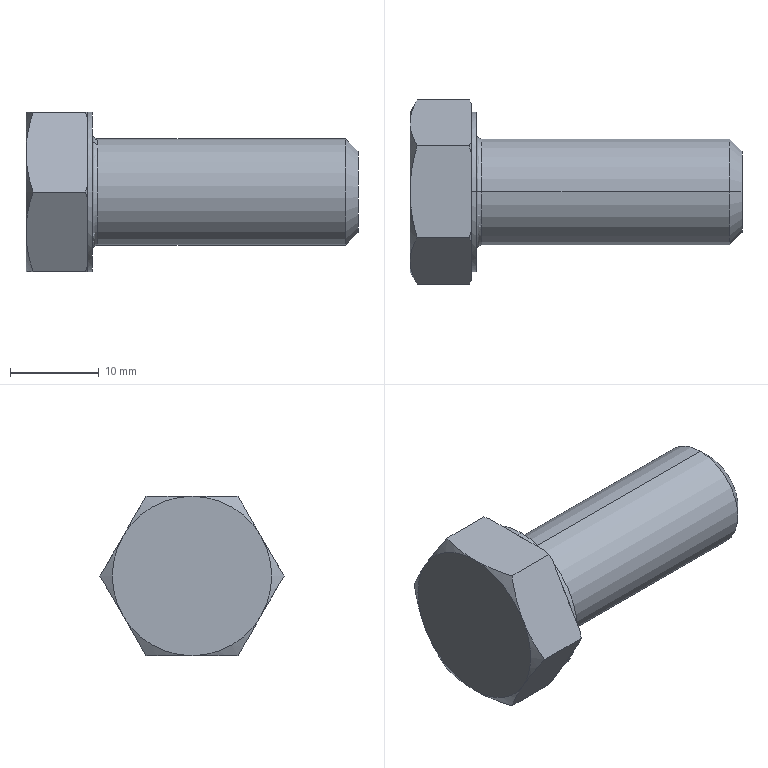Part | SolidWorks | features RevCut 4, Chamfer 1, Extrusion 1, Fillet 1, LPattern 1, Revolution 1 | 1 solid | 35 faces | box 37.5 x 20.785 x 18 mm | volume 5444 mm3 | plane 15 | cone 14 | cylinder 4 | torus 2 | commonest cylinder face diameters 12 x2 18 x2
STEP:
#1=CARTESIAN_POINT('',(8.1,0.,6.));
#2=VERTEX_POINT('',#1);
#3=CARTESIAN_POINT('',(8.1,0.,-6.));
#4=VERTEX_POINT('',#3);
#5=CARTESIAN_POINT('',(8.1,0.,0.));
#6=DIRECTION('',(1.,0.,0.));
#7=DIRECTION('',(0.,0.,-1.));
#8=AXIS2_PLACEMENT_3D('',#5,#6,#7);
#9=CIRCLE('',#8,6.);
#10=EDGE_CURVE('',#2,#4,#9,.T.);
#11=ORIENTED_EDGE('',*,*,#10,.F.);
#12=CARTESIAN_POINT('',(7.5,0.,6.6));
#13=VERTEX_POINT('',#12);
#14=CARTESIAN_POINT('',(8.1,0.,6.6));
#15=DIRECTION('',(0.,1.,0.));
#16=DIRECTION('',(0.,0.,1.));
#17=AXIS2_PLACEMENT_3D('',#14,#15,#16);
#18=CIRCLE('',#17,0.6);
#19=EDGE_CURVE('',#2,#13,#18,.T.);
#20=ORIENTED_EDGE('',*,*,#19,.T.);
#21=CARTESIAN_POINT('',(7.5,0.,-6.6));
#22=VERTEX_POINT('',#21);
#23=CARTESIAN_POINT('',(7.5,0.,0.));
#24=DIRECTION('',(-1.,0.,0.));
#25=DIRECTION('',(0.,0.,-1.));
#26=AXIS2_PLACEMENT_3D('',#23,#24,#25);
#27=CIRCLE('',#26,6.6);
#28=EDGE_CURVE('',#22,#13,#27,.T.);
#29=ORIENTED_EDGE('',*,*,#28,.F.);
#30=CARTESIAN_POINT('',(8.1,0.,-6.6));
#31=DIRECTION('',(0.,-1.,0.));
#32=DIRECTION('',(0.,0.,-1.));
#33=AXIS2_PLACEMENT_3D('',#30,#31,#32);
#34=CIRCLE('',#33,0.6);
#35=EDGE_CURVE('',#4,#22,#34,.T.);
#36=ORIENTED_EDGE('',*,*,#35,.F.);
#37=EDGE_LOOP('',(#11,#20,#29,#36));
#38=FACE_OUTER_BOUND('',#37,.T.);
#39=CARTESIAN_POINT('',(8.1,0.,0.));
#40=DIRECTION('',(1.,0.,0.));
#41=DIRECTION('',(0.,0.,-1.));
#42=AXIS2_PLACEMENT_3D('',#39,#40,#41);
#43=TOROIDAL_SURFACE('',#42,6.6,0.6);
#44=ADVANCED_FACE('',(#38),#43,.F.);
#45=CARTESIAN_POINT('',(37.5,0.,-4.6));
#46=VERTEX_POINT('',#45);
#47=CARTESIAN_POINT('',(37.5,0.,4.6));
#48=VERTEX_POINT('',#47);
#49=CARTESIAN_POINT('',(37.5,0.,0.));
#50=DIRECTION('',(1.,0.,0.));
#51=DIRECTION('',(0.,0.,1.));
#52=AXIS2_PLACEMENT_3D('',#49,#50,#51);
#53=CIRCLE('',#52,4.6);
#54=EDGE_CURVE('',#46,#48,#53,.T.);
#55=ORIENTED_EDGE('',*,*,#54,.F.);
#56=CARTESIAN_POINT('',(36.1,0.,-6.));
#57=VERTEX_POINT('',#56);
#58=CARTESIAN_POINT('',(36.1,0.,-6.));
#59=DIRECTION('',(-0.7071,0.,-0.7071));
#60=VECTOR('',#59,1000.);
#61=LINE('',#58,#60);
#62=EDGE_CURVE('',#46,#57,#61,.T.);
#63=ORIENTED_EDGE('',*,*,#62,.T.);
#64=CARTESIAN_POINT('',(36.1,0.,6.));
#65=VERTEX_POINT('',#64);
#66=CARTESIAN_POINT('',(36.1,0.,0.));
#67=DIRECTION('',(-1.,0.,0.));
#68=DIRECTION('',(0.,0.,1.));
#69=AXIS2_PLACEMENT_3D('',#66,#67,#68);
#70=CIRCLE('',#69,6.);
#71=EDGE_CURVE('',#65,#57,#70,.T.);
#72=ORIENTED_EDGE('',*,*,#71,.F.);
#73=CARTESIAN_POINT('',(36.1,0.,6.));
#74=DIRECTION('',(-0.7071,0.,0.7071));
#75=VECTOR('',#74,1000.);
#76=LINE('',#73,#75);
#77=EDGE_CURVE('',#48,#65,#76,.T.);
#78=ORIENTED_EDGE('',*,*,#77,.F.);
#79=EDGE_LOOP('',(#55,#63,#72,#78));
#80=FACE_OUTER_BOUND('',#79,.T.);
#81=CARTESIAN_POINT('',(36.1,0.,0.));
#82=DIRECTION('',(-1.,0.,0.));
#83=DIRECTION('',(0.,0.,1.));
#84=AXIS2_PLACEMENT_3D('',#81,#82,#83);
#85=CONICAL_SURFACE('',#84,6.,0.7854);
#86=ADVANCED_FACE('',(#80),#85,.T.);
#87=ORIENTED_EDGE('',*,*,#71,.T.);
#88=CARTESIAN_POINT('',(0.,0.,-6.));
#89=DIRECTION('',(-1.,0.,0.));
#90=VECTOR('',#89,1000.);
#91=LINE('',#88,#90);
#92=EDGE_CURVE('',#57,#4,#91,.T.);
#93=ORIENTED_EDGE('',*,*,#92,.T.);
#94=CARTESIAN_POINT('',(8.1,0.,0.));
#95=DIRECTION('',(1.,0.,0.));
#96=DIRECTION('',(0.,0.,-1.));
#97=AXIS2_PLACEMENT_3D('',#94,#95,#96);
#98=CIRCLE('',#97,6.);
#99=EDGE_CURVE('',#4,#2,#98,.T.);
#100=ORIENTED_EDGE('',*,*,#99,.T.);
#101=CARTESIAN_POINT('',(0.,0.,6.));
#102=DIRECTION('',(-1.,0.,0.));
#103=VECTOR('',#102,1000.);
#104=LINE('',#101,#103);
#105=EDGE_CURVE('',#65,#2,#104,.T.);
#106=ORIENTED_EDGE('',*,*,#105,.F.);
#107=EDGE_LOOP('',(#87,#93,#100,#106));
#108=FACE_OUTER_BOUND('',#107,.T.);
#109=CARTESIAN_POINT('',(0.,0.,0.));
#110=DIRECTION('',(-1.,0.,0.));
#111=DIRECTION('',(0.,0.,1.));
#112=AXIS2_PLACEMENT_3D('',#109,#110,#111);
#113=CYLINDRICAL_SURFACE('',#112,6.);
#114=ADVANCED_FACE('',(#108),#113,.T.);
#115=CARTESIAN_POINT('',(7.5,0.,-9.));
#116=VERTEX_POINT('',#115);
#117=CARTESIAN_POINT('',(7.5,0.,9.));
#118=VERTEX_POINT('',#117);
#119=CARTESIAN_POINT('',(7.5,0.,0.));
#120=DIRECTION('',(1.,0.,0.));
#121=DIRECTION('',(0.,0.,-1.));
#122=AXIS2_PLACEMENT_3D('',#119,#120,#121);
#123=CIRCLE('',#122,9.);
#124=EDGE_CURVE('',#116,#118,#123,.T.);
#125=ORIENTED_EDGE('',*,*,#124,.F.);
#126=CARTESIAN_POINT('',(6.9,0.,-9.));
#127=VERTEX_POINT('',#126);
#128=CARTESIAN_POINT('',(0.,0.,-9.));
#129=DIRECTION('',(-1.,0.,0.));
#130=VECTOR('',#129,1000.);
#131=LINE('',#128,#130);
#132=EDGE_CURVE('',#116,#127,#131,.T.);
#133=ORIENTED_EDGE('',*,*,#132,.T.);
#134=CARTESIAN_POINT('',(6.9,7.794,-4.5));
#135=VERTEX_POINT('',#134);
#136=CARTESIAN_POINT('',(6.9,0.,0.));
#137=DIRECTION('',(-1.,0.,0.));
#138=DIRECTION('',(0.,0.,1.));
#139=AXIS2_PLACEMENT_3D('',#136,#137,#138);
#140=CIRCLE('',#139,9.);
#141=EDGE_CURVE('',#135,#127,#140,.T.);
#142=ORIENTED_EDGE('',*,*,#141,.F.);
#143=CARTESIAN_POINT('',(6.9,7.794,4.5));
#144=VERTEX_POINT('',#143);
#145=CARTESIAN_POINT('',(6.9,0.,0.));
#146=DIRECTION('',(-1.,0.,0.));
#147=DIRECTION('',(0.,0.,1.));
#148=AXIS2_PLACEMENT_3D('',#145,#146,#147);
#149=CIRCLE('',#148,9.);
#150=EDGE_CURVE('',#144,#135,#149,.T.);
#151=ORIENTED_EDGE('',*,*,#150,.F.);
#152=CARTESIAN_POINT('',(6.9,0.,9.));
#153=VERTEX_POINT('',#152);
#154=CARTESIAN_POINT('',(6.9,0.,0.));
#155=DIRECTION('',(-1.,0.,0.));
#156=DIRECTION('',(0.,0.,1.));
#157=AXIS2_PLACEMENT_3D('',#154,#155,#156);
#158=CIRCLE('',#157,9.);
#159=EDGE_CURVE('',#153,#144,#158,.T.);
#160=ORIENTED_EDGE('',*,*,#159,.F.);
#161=CARTESIAN_POINT('',(0.,0.,9.));
#162=DIRECTION('',(-1.,0.,0.));
#163=VECTOR('',#162,1000.);
#164=LINE('',#161,#163);
#165=EDGE_CURVE('',#118,#153,#164,.T.);
#166=ORIENTED_EDGE('',*,*,#165,.F.);
#167=EDGE_LOOP('',(#125,#133,#142,#151,#160,#166));
#168=FACE_OUTER_BOUND('',#167,.T.);
#169=CARTESIAN_POINT('',(0.,0.,0.));
#170=DIRECTION('',(-1.,0.,0.));
#171=DIRECTION('',(0.,0.,1.));
#172=AXIS2_PLACEMENT_3D('',#169,#170,#171);
#173=CYLINDRICAL_SURFACE('',#172,9.);
#174=ADVANCED_FACE('',(#168),#173,.T.);
#175=CARTESIAN_POINT('',(6.9,5.57,-8.352));
#176=VERTEX_POINT('',#175);
#177=CARTESIAN_POINT('',(6.9,5.196,-9.));
#178=DIRECTION('',(0.,0.5,0.866));
#179=VECTOR('',#178,1000.);
#180=LINE('',#177,#179);
#181=EDGE_CURVE('',#176,#135,#180,.T.);
#182=ORIENTED_EDGE('',*,*,#181,.F.);
#183=CARTESIAN_POINT('',(6.696,5.196,-9.));
#184=VERTEX_POINT('',#183);
#185=CARTESIAN_POINT('',(6.696,5.196,-9.));
#186=CARTESIAN_POINT('',(6.768,5.321,-8.785));
#187=CARTESIAN_POINT('',(6.836,5.445,-8.569));
#188=CARTESIAN_POINT('',(6.9,5.57,-8.352));
#189=B_SPLINE_CURVE_WITH_KNOTS('',3,(#185,#186,#187,#188),.UNSPECIFIED.,.F.,.F.,(4,4),(0.000000238,0.0007696),.UNSPECIFIED.);
#190=EDGE_CURVE('',#184,#176,#189,.T.);
#191=ORIENTED_EDGE('',*,*,#190,.F.);
#192=CARTESIAN_POINT('',(0.8038,5.196,-9.));
#193=VERTEX_POINT('',#192);
#194=CARTESIAN_POINT('',(7.5,5.196,-9.));
#195=DIRECTION('',(-1.,0.,0.));
#196=VECTOR('',#195,1000.);
#197=LINE('',#194,#196);
#198=EDGE_CURVE('',#184,#193,#197,.T.);
#199=ORIENTED_EDGE('',*,*,#198,.T.);
#200=CARTESIAN_POINT('',(0.,7.794,-4.5));
#201=VERTEX_POINT('',#200);
#202=CARTESIAN_POINT('',(0.,7.794,-4.5));
#203=CARTESIAN_POINT('',(0.,7.574,-4.882));
#204=CARTESIAN_POINT('',(0.019,7.352,-5.266));
#205=CARTESIAN_POINT('',(0.09253,6.914,-6.024));
#206=CARTESIAN_POINT('',(0.147,6.697,-6.401));
#207=CARTESIAN_POINT('',(0.357,6.048,-7.525));
#208=CARTESIAN_POINT('',(0.5591,5.62,-8.266));
#209=CARTESIAN_POINT('',(0.8038,5.196,-9.));
#210=B_SPLINE_CURVE_WITH_KNOTS('',3,(#202,#203,#204,#205,#206,#207,#208,#209),.UNSPECIFIED.,.F.,.F.,(4,2,2,4),(0.005258,0.006567,0.007877,0.0105),.UNSPECIFIED.);
#211=EDGE_CURVE('',#201,#193,#210,.T.);
#212=ORIENTED_EDGE('',*,*,#211,.F.);
#213=CARTESIAN_POINT('',(0.8038,10.392,0.));
#214=VERTEX_POINT('',#213);
#215=CARTESIAN_POINT('',(0.8038,10.392,0.));
#216=CARTESIAN_POINT('',(0.5585,9.967,-0.7361));
#217=CARTESIAN_POINT('',(0.3563,9.539,-1.478));
#218=CARTESIAN_POINT('',(0.07661,8.674,-2.976));
#219=CARTESIAN_POINT('',(0.,8.237,-3.733));
#220=CARTESIAN_POINT('',(0.,7.794,-4.5));
#221=B_SPLINE_CURVE_WITH_KNOTS('',3,(#215,#216,#217,#218,#219,#220),.UNSPECIFIED.,.F.,.F.,(4,2,4),(0.000000238,0.002629,0.005258),.UNSPECIFIED.);
#222=EDGE_CURVE('',#214,#201,#221,.T.);
#223=ORIENTED_EDGE('',*,*,#222,.F.);
#224=CARTESIAN_POINT('',(6.696,10.392,0.));
#225=VERTEX_POINT('',#224);
#226=CARTESIAN_POINT('',(7.5,10.392,0.));
#227=DIRECTION('',(-1.,0.,0.));
#228=VECTOR('',#227,1000.);
#229=LINE('',#226,#228);
#230=EDGE_CURVE('',#225,#214,#229,.T.);
#231=ORIENTED_EDGE('',*,*,#230,.F.);
#232=CARTESIAN_POINT('',(6.9,10.018,-0.6478));
#233=VERTEX_POINT('',#232);
#234=CARTESIAN_POINT('',(6.9,10.018,-0.6478));
#235=CARTESIAN_POINT('',(6.836,10.143,-0.4313));
#236=CARTESIAN_POINT('',(6.768,10.268,-0.2154));
#237=CARTESIAN_POINT('',(6.696,10.392,0.));
#238=B_SPLINE_CURVE_WITH_KNOTS('',3,(#234,#235,#236,#237),.UNSPECIFIED.,.F.,.F.,(4,4),(0.009728,0.0105),.UNSPECIFIED.);
#239=EDGE_CURVE('',#233,#225,#238,.T.);
#240=ORIENTED_EDGE('',*,*,#239,.F.);
#241=CARTESIAN_POINT('',(6.9,5.196,-9.));
#242=DIRECTION('',(0.,0.5,0.866));
#243=VECTOR('',#242,1000.);
#244=LINE('',#241,#243);
#245=EDGE_CURVE('',#135,#233,#244,.T.);
#246=ORIENTED_EDGE('',*,*,#245,.F.);
#247=EDGE_LOOP('',(#182,#191,#199,#212,#223,#231,#240,#246));
#248=FACE_OUTER_BOUND('',#247,.T.);
#249=CARTESIAN_POINT('',(7.5,5.196,-9.));
#250=DIRECTION('',(0.,-0.866,0.5));
#251=DIRECTION('',(0.,-0.5,-0.866));
#252=AXIS2_PLACEMENT_3D('',#249,#250,#251);
#253=PLANE('',#252);
#254=ADVANCED_FACE('',(#248),#253,.F.);
#255=CARTESIAN_POINT('',(6.9,10.018,0.6478));
#256=VERTEX_POINT('',#255);
#257=CARTESIAN_POINT('',(6.9,10.392,0.));
#258=DIRECTION('',(0.,-0.5,0.866));
#259=VECTOR('',#258,1000.);
#260=LINE('',#257,#259);
#261=EDGE_CURVE('',#256,#144,#260,.T.);
#262=ORIENTED_EDGE('',*,*,#261,.F.);
#263=CARTESIAN_POINT('',(6.696,10.392,0.));
#264=CARTESIAN_POINT('',(6.768,10.268,0.2154));
#265=CARTESIAN_POINT('',(6.836,10.143,0.4314));
#266=CARTESIAN_POINT('',(6.9,10.018,0.6478));
#267=B_SPLINE_CURVE_WITH_KNOTS('',3,(#263,#264,#265,#266),.UNSPECIFIED.,.F.,.F.,(4,4),(0.000000238,0.0007696),.UNSPECIFIED.);
#268=EDGE_CURVE('',#225,#256,#267,.T.);
#269=ORIENTED_EDGE('',*,*,#268,.F.);
#270=ORIENTED_EDGE('',*,*,#230,.T.);
#271=CARTESIAN_POINT('',(0.,7.794,4.5));
#272=VERTEX_POINT('',#271);
#273=CARTESIAN_POINT('',(0.,7.794,4.5));
#274=CARTESIAN_POINT('',(0.,8.015,4.118));
#275=CARTESIAN_POINT('',(0.019,8.236,3.734));
#276=CARTESIAN_POINT('',(0.09253,8.674,2.976));
#277=CARTESIAN_POINT('',(0.147,8.892,2.599));
#278=CARTESIAN_POINT('',(0.357,9.541,1.475));
#279=CARTESIAN_POINT('',(0.5591,9.968,0.7343));
#280=CARTESIAN_POINT('',(0.8038,10.392,0.));
#281=B_SPLINE_CURVE_WITH_KNOTS('',3,(#273,#274,#275,#276,#277,#278,#279,#280),.UNSPECIFIED.,.F.,.F.,(4,2,2,4),(0.005258,0.006567,0.007877,0.0105),.UNSPECIFIED.);
#282=EDGE_CURVE('',#272,#214,#281,.T.);
#283=ORIENTED_EDGE('',*,*,#282,.F.);
#284=CARTESIAN_POINT('',(0.8038,5.196,9.));
#285=VERTEX_POINT('',#284);
#286=CARTESIAN_POINT('',(0.8038,5.196,9.));
#287=CARTESIAN_POINT('',(0.5585,5.621,8.264));
#288=CARTESIAN_POINT('',(0.3563,6.049,7.522));
#289=CARTESIAN_POINT('',(0.07661,6.914,6.024));
#290=CARTESIAN_POINT('',(0.,7.352,5.267));
#291=CARTESIAN_POINT('',(0.,7.794,4.5));
#292=B_SPLINE_CURVE_WITH_KNOTS('',3,(#286,#287,#288,#289,#290,#291),.UNSPECIFIED.,.F.,.F.,(4,2,4),(0.000000238,0.002629,0.005258),.UNSPECIFIED.);
#293=EDGE_CURVE('',#285,#272,#292,.T.);
#294=ORIENTED_EDGE('',*,*,#293,.F.);
#295=CARTESIAN_POINT('',(6.696,5.196,9.));
#296=VERTEX_POINT('',#295);
#297=CARTESIAN_POINT('',(7.5,5.196,9.));
#298=DIRECTION('',(-1.,0.,0.));
#299=VECTOR('',#298,1000.);
#300=LINE('',#297,#299);
#301=EDGE_CURVE('',#296,#285,#300,.T.);
#302=ORIENTED_EDGE('',*,*,#301,.F.);
#303=CARTESIAN_POINT('',(6.9,5.57,8.352));
#304=VERTEX_POINT('',#303);
#305=CARTESIAN_POINT('',(6.9,5.57,8.352));
#306=CARTESIAN_POINT('',(6.836,5.445,8.569));
#307=CARTESIAN_POINT('',(6.768,5.32,8.785));
#308=CARTESIAN_POINT('',(6.696,5.196,9.));
#309=B_SPLINE_CURVE_WITH_KNOTS('',3,(#305,#306,#307,#308),.UNSPECIFIED.,.F.,.F.,(4,4),(0.009728,0.0105),.UNSPECIFIED.);
#310=EDGE_CURVE('',#304,#296,#309,.T.);
#311=ORIENTED_EDGE('',*,*,#310,.F.);
#312=CARTESIAN_POINT('',(6.9,10.392,0.));
#313=DIRECTION('',(0.,-0.5,0.866));
#314=VECTOR('',#313,1000.);
#315=LINE('',#312,#314);
#316=EDGE_CURVE('',#144,#304,#315,.T.);
#317=ORIENTED_EDGE('',*,*,#316,.F.);
#318=EDGE_LOOP('',(#262,#269,#270,#283,#294,#302,#311,#317));
#319=FACE_OUTER_BOUND('',#318,.T.);
#320=CARTESIAN_POINT('',(7.5,10.392,0.));
#321=DIRECTION('',(0.,-0.866,-0.5));
#322=DIRECTION('',(0.,0.5,-0.866));
#323=AXIS2_PLACEMENT_3D('',#320,#321,#322);
#324=PLANE('',#323);
#325=ADVANCED_FACE('',(#319),#324,.F.);
#326=CARTESIAN_POINT('',(6.9,4.448,9.));
#327=VERTEX_POINT('',#326);
#328=CARTESIAN_POINT('',(6.9,5.196,9.));
#329=DIRECTION('',(0.,-1.,0.));
#330=VECTOR('',#329,1000.);
#331=LINE('',#328,#330);
#332=EDGE_CURVE('',#327,#153,#331,.T.);
#333=ORIENTED_EDGE('',*,*,#332,.F.);
#334=CARTESIAN_POINT('',(6.696,5.196,9.));
#335=CARTESIAN_POINT('',(6.768,4.948,9.));
#336=CARTESIAN_POINT('',(6.836,4.698,9.));
#337=CARTESIAN_POINT('',(6.9,4.448,9.));
#338=B_SPLINE_CURVE_WITH_KNOTS('',3,(#334,#335,#336,#337),.UNSPECIFIED.,.F.,.F.,(4,4),(0.02519,0.02597),.UNSPECIFIED.);
#339=EDGE_CURVE('',#296,#327,#338,.T.);
#340=ORIENTED_EDGE('',*,*,#339,.F.);
#341=ORIENTED_EDGE('',*,*,#301,.T.);
#342=CARTESIAN_POINT('',(0.,0.,9.));
#343=VERTEX_POINT('',#342);
#344=CARTESIAN_POINT('',(0.,0.,9.));
#345=CARTESIAN_POINT('',(0.,0.4401,9.));
#346=CARTESIAN_POINT('',(0.01885,0.8832,9.));
#347=CARTESIAN_POINT('',(0.09319,1.767,9.));
#348=CARTESIAN_POINT('',(0.1482,2.204,9.));
#349=CARTESIAN_POINT('',(0.3593,3.505,9.));
#350=CARTESIAN_POINT('',(0.5612,4.356,9.));
#351=CARTESIAN_POINT('',(0.8038,5.196,9.));
#352=B_SPLINE_CURVE_WITH_KNOTS('',3,(#344,#345,#346,#347,#348,#349,#350,#351),.UNSPECIFIED.,.F.,.F.,(4,2,2,4),(0.01498,0.0163,0.01761,0.02025),.UNSPECIFIED.);
#353=EDGE_CURVE('',#343,#285,#352,.T.);
#354=ORIENTED_EDGE('',*,*,#353,.F.);
#355=CARTESIAN_POINT('',(0.8038,-5.196,9.));
#356=VERTEX_POINT('',#355);
#357=CARTESIAN_POINT('',(0.8038,-5.196,9.));
#358=CARTESIAN_POINT('',(0.5595,-4.35,9.));
#359=CARTESIAN_POINT('',(0.3552,-3.485,9.));
#360=CARTESIAN_POINT('',(0.07569,-1.752,9.));
#361=CARTESIAN_POINT('',(0.,-0.8794,9.));
#362=CARTESIAN_POINT('',(0.,0.,9.));
#363=B_SPLINE_CURVE_WITH_KNOTS('',3,(#357,#358,#359,#360,#361,#362),.UNSPECIFIED.,.F.,.F.,(4,2,4),(0.00972,0.01235,0.01498),.UNSPECIFIED.);
#364=EDGE_CURVE('',#356,#343,#363,.T.);
#365=ORIENTED_EDGE('',*,*,#364,.F.);
#366=CARTESIAN_POINT('',(6.696,-5.196,9.));
#367=VERTEX_POINT('',#366);
#368=CARTESIAN_POINT('',(7.5,-5.196,9.));
#369=DIRECTION('',(-1.,0.,0.));
#370=VECTOR('',#369,1000.);
#371=LINE('',#368,#370);
#372=EDGE_CURVE('',#367,#356,#371,.T.);
#373=ORIENTED_EDGE('',*,*,#372,.F.);
#374=CARTESIAN_POINT('',(6.9,-4.448,9.));
#375=VERTEX_POINT('',#374);
#376=CARTESIAN_POINT('',(6.9,-4.448,9.));
#377=CARTESIAN_POINT('',(6.836,-4.699,9.));
#378=CARTESIAN_POINT('',(6.768,-4.948,9.));
#379=CARTESIAN_POINT('',(6.696,-5.196,9.));
#380=B_SPLINE_CURVE_WITH_KNOTS('',3,(#376,#377,#378,#379),.UNSPECIFIED.,.F.,.F.,(4,4),(0.03494,0.03571),.UNSPECIFIED.);
#381=EDGE_CURVE('',#375,#367,#380,.T.);
#382=ORIENTED_EDGE('',*,*,#381,.F.);
#383=CARTESIAN_POINT('',(6.9,5.196,9.));
#384=DIRECTION('',(0.,-1.,0.));
#385=VECTOR('',#384,1000.);
#386=LINE('',#383,#385);
#387=EDGE_CURVE('',#153,#375,#386,.T.);
#388=ORIENTED_EDGE('',*,*,#387,.F.);
#389=EDGE_LOOP('',(#333,#340,#341,#354,#365,#373,#382,#388));
#390=FACE_OUTER_BOUND('',#389,.T.);
#391=CARTESIAN_POINT('',(7.5,5.196,9.));
#392=DIRECTION('',(0.,0.,-1.));
#393=DIRECTION('',(0.,1.,0.));
#394=AXIS2_PLACEMENT_3D('',#391,#392,#393);
#395=PLANE('',#394);
#396=ADVANCED_FACE('',(#390),#395,.F.);
#397=CARTESIAN_POINT('',(6.9,-5.57,8.352));
#398=VERTEX_POINT('',#397);
#399=CARTESIAN_POINT('',(6.9,-7.794,4.5));
#400=VERTEX_POINT('',#399);
#401=CARTESIAN_POINT('',(6.9,-10.392,0.));
#402=DIRECTION('',(0.,-0.5,-0.866));
#403=VECTOR('',#402,1000.);
#404=LINE('',#401,#403);
#405=EDGE_CURVE('',#398,#400,#404,.T.);
#406=ORIENTED_EDGE('',*,*,#405,.F.);
#407=CARTESIAN_POINT('',(6.696,-5.196,9.));
#408=CARTESIAN_POINT('',(6.768,-5.321,8.785));
#409=CARTESIAN_POINT('',(6.836,-5.445,8.569));
#410=CARTESIAN_POINT('',(6.9,-5.57,8.352));
#411=B_SPLINE_CURVE_WITH_KNOTS('',3,(#407,#408,#409,#410),.UNSPECIFIED.,.F.,.F.,(4,4),(0.000000238,0.0007696),.UNSPECIFIED.);
#412=EDGE_CURVE('',#367,#398,#411,.T.);
#413=ORIENTED_EDGE('',*,*,#412,.F.);
#414=ORIENTED_EDGE('',*,*,#372,.T.);
#415=CARTESIAN_POINT('',(0.,-7.794,4.5));
#416=VERTEX_POINT('',#415);
#417=CARTESIAN_POINT('',(0.,-7.794,4.5));
#418=CARTESIAN_POINT('',(0.,-7.574,4.882));
#419=CARTESIAN_POINT('',(0.019,-7.352,5.266));
#420=CARTESIAN_POINT('',(0.09253,-6.914,6.024));
#421=CARTESIAN_POINT('',(0.147,-6.697,6.401));
#422=CARTESIAN_POINT('',(0.357,-6.048,7.525));
#423=CARTESIAN_POINT('',(0.5591,-5.62,8.266));
#424=CARTESIAN_POINT('',(0.8038,-5.196,9.));
#425=B_SPLINE_CURVE_WITH_KNOTS('',3,(#417,#418,#419,#420,#421,#422,#423,#424),.UNSPECIFIED.,.F.,.F.,(4,2,2,4),(0.005258,0.006567,0.007877,0.0105),.UNSPECIFIED.);
#426=EDGE_CURVE('',#416,#356,#425,.T.);
#427=ORIENTED_EDGE('',*,*,#426,.F.);
#428=CARTESIAN_POINT('',(0.8038,-10.392,0.));
#429=VERTEX_POINT('',#428);
#430=CARTESIAN_POINT('',(0.8038,-10.392,0.));
#431=CARTESIAN_POINT('',(0.5585,-9.967,0.7361));
#432=CARTESIAN_POINT('',(0.3563,-9.539,1.478));
#433=CARTESIAN_POINT('',(0.07661,-8.674,2.976));
#434=CARTESIAN_POINT('',(0.,-8.237,3.733));
#435=CARTESIAN_POINT('',(0.,-7.794,4.5));
#436=B_SPLINE_CURVE_WITH_KNOTS('',3,(#430,#431,#432,#433,#434,#435),.UNSPECIFIED.,.F.,.F.,(4,2,4),(0.000000238,0.002629,0.005258),.UNSPECIFIED.);
#437=EDGE_CURVE('',#429,#416,#436,.T.);
#438=ORIENTED_EDGE('',*,*,#437,.F.);
#439=CARTESIAN_POINT('',(6.696,-10.392,0.));
#440=VERTEX_POINT('',#439);
#441=CARTESIAN_POINT('',(7.5,-10.392,0.));
#442=DIRECTION('',(-1.,0.,0.));
#443=VECTOR('',#442,1000.);
#444=LINE('',#441,#443);
#445=EDGE_CURVE('',#440,#429,#444,.T.);
#446=ORIENTED_EDGE('',*,*,#445,.F.);
#447=CARTESIAN_POINT('',(6.9,-10.018,0.6478));
#448=VERTEX_POINT('',#447);
#449=CARTESIAN_POINT('',(6.9,-10.018,0.6478));
#450=CARTESIAN_POINT('',(6.836,-10.143,0.4313));
#451=CARTESIAN_POINT('',(6.768,-10.268,0.2154));
#452=CARTESIAN_POINT('',(6.696,-10.392,0.));
#453=B_SPLINE_CURVE_WITH_KNOTS('',3,(#449,#450,#451,#452),.UNSPECIFIED.,.F.,.F.,(4,4),(0.009728,0.0105),.UNSPECIFIED.);
#454=EDGE_CURVE('',#448,#440,#453,.T.);
#455=ORIENTED_EDGE('',*,*,#454,.F.);
#456=CARTESIAN_POINT('',(6.9,-10.392,0.));
#457=DIRECTION('',(0.,-0.5,-0.866));
#458=VECTOR('',#457,1000.);
#459=LINE('',#456,#458);
#460=EDGE_CURVE('',#400,#448,#459,.T.);
#461=ORIENTED_EDGE('',*,*,#460,.F.);
#462=EDGE_LOOP('',(#406,#413,#414,#427,#438,#446,#455,#461));
#463=FACE_OUTER_BOUND('',#462,.T.);
#464=CARTESIAN_POINT('',(7.5,-10.392,0.));
#465=DIRECTION('',(0.,0.866,-0.5));
#466=DIRECTION('',(0.,0.5,0.866));
#467=AXIS2_PLACEMENT_3D('',#464,#465,#466);
#468=PLANE('',#467);
#469=ADVANCED_FACE('',(#463),#468,.F.);
#470=CARTESIAN_POINT('',(6.9,-10.018,-0.6478));
#471=VERTEX_POINT('',#470);
#472=CARTESIAN_POINT('',(6.9,-7.794,-4.5));
#473=VERTEX_POINT('',#472);
#474=CARTESIAN_POINT('',(6.9,-5.196,-9.));
#475=DIRECTION('',(0.,0.5,-0.866));
#476=VECTOR('',#475,1000.);
#477=LINE('',#474,#476);
#478=EDGE_CURVE('',#471,#473,#477,.T.);
#479=ORIENTED_EDGE('',*,*,#478,.F.);
#480=CARTESIAN_POINT('',(6.696,-10.392,0.));
#481=CARTESIAN_POINT('',(6.768,-10.268,-0.2154));
#482=CARTESIAN_POINT('',(6.836,-10.143,-0.4314));
#483=CARTESIAN_POINT('',(6.9,-10.018,-0.6478));
#484=B_SPLINE_CURVE_WITH_KNOTS('',3,(#480,#481,#482,#483),.UNSPECIFIED.,.F.,.F.,(4,4),(0.000000238,0.0007696),.UNSPECIFIED.);
#485=EDGE_CURVE('',#440,#471,#484,.T.);
#486=ORIENTED_EDGE('',*,*,#485,.F.);
#487=ORIENTED_EDGE('',*,*,#445,.T.);
#488=CARTESIAN_POINT('',(0.,-7.794,-4.5));
#489=VERTEX_POINT('',#488);
#490=CARTESIAN_POINT('',(0.,-7.794,-4.5));
#491=CARTESIAN_POINT('',(0.,-8.015,-4.118));
#492=CARTESIAN_POINT('',(0.019,-8.236,-3.734));
#493=CARTESIAN_POINT('',(0.09253,-8.674,-2.976));
#494=CARTESIAN_POINT('',(0.147,-8.892,-2.599));
#495=CARTESIAN_POINT('',(0.357,-9.541,-1.475));
#496=CARTESIAN_POINT('',(0.5591,-9.968,-0.7343));
#497=CARTESIAN_POINT('',(0.8038,-10.392,0.));
#498=B_SPLINE_CURVE_WITH_KNOTS('',3,(#490,#491,#492,#493,#494,#495,#496,#497),.UNSPECIFIED.,.F.,.F.,(4,2,2,4),(0.005258,0.006567,0.007877,0.0105),.UNSPECIFIED.);
#499=EDGE_CURVE('',#489,#429,#498,.T.);
#500=ORIENTED_EDGE('',*,*,#499,.F.);
#501=CARTESIAN_POINT('',(0.8038,-5.196,-9.));
#502=VERTEX_POINT('',#501);
#503=CARTESIAN_POINT('',(0.8038,-5.196,-9.));
#504=CARTESIAN_POINT('',(0.5585,-5.621,-8.264));
#505=CARTESIAN_POINT('',(0.3563,-6.049,-7.522));
#506=CARTESIAN_POINT('',(0.07661,-6.914,-6.024));
#507=CARTESIAN_POINT('',(0.,-7.352,-5.267));
#508=CARTESIAN_POINT('',(0.,-7.794,-4.5));
#509=B_SPLINE_CURVE_WITH_KNOTS('',3,(#503,#504,#505,#506,#507,#508),.UNSPECIFIED.,.F.,.F.,(4,2,4),(0.000000238,0.002629,0.005258),.UNSPECIFIED.);
#510=EDGE_CURVE('',#502,#489,#509,.T.);
#511=ORIENTED_EDGE('',*,*,#510,.F.);
#512=CARTESIAN_POINT('',(6.696,-5.196,-9.));
#513=VERTEX_POINT('',#512);
#514=CARTESIAN_POINT('',(7.5,-5.196,-9.));
#515=DIRECTION('',(-1.,0.,0.));
#516=VECTOR('',#515,1000.);
#517=LINE('',#514,#516);
#518=EDGE_CURVE('',#513,#502,#517,.T.);
#519=ORIENTED_EDGE('',*,*,#518,.F.);
#520=CARTESIAN_POINT('',(6.9,-5.57,-8.352));
#521=VERTEX_POINT('',#520);
#522=CARTESIAN_POINT('',(6.9,-5.57,-8.352));
#523=CARTESIAN_POINT('',(6.836,-5.445,-8.569));
#524=CARTESIAN_POINT('',(6.768,-5.32,-8.785));
#525=CARTESIAN_POINT('',(6.696,-5.196,-9.));
#526=B_SPLINE_CURVE_WITH_KNOTS('',3,(#522,#523,#524,#525),.UNSPECIFIED.,.F.,.F.,(4,4),(0.009728,0.0105),.UNSPECIFIED.);
#527=EDGE_CURVE('',#521,#513,#526,.T.);
#528=ORIENTED_EDGE('',*,*,#527,.F.);
#529=CARTESIAN_POINT('',(6.9,-5.196,-9.));
#530=DIRECTION('',(0.,0.5,-0.866));
#531=VECTOR('',#530,1000.);
#532=LINE('',#529,#531);
#533=EDGE_CURVE('',#473,#521,#532,.T.);
#534=ORIENTED_EDGE('',*,*,#533,.F.);
#535=EDGE_LOOP('',(#479,#486,#487,#500,#511,#519,#528,#534));
#536=FACE_OUTER_BOUND('',#535,.T.);
#537=CARTESIAN_POINT('',(7.5,-5.196,-9.));
#538=DIRECTION('',(0.,0.866,0.5));
#539=DIRECTION('',(0.,-0.5,0.866));
#540=AXIS2_PLACEMENT_3D('',#537,#538,#539);
#541=PLANE('',#540);
#542=ADVANCED_FACE('',(#536),#541,.F.);
#543=CARTESIAN_POINT('',(6.9,-4.448,-9.));
#544=VERTEX_POINT('',#543);
#545=CARTESIAN_POINT('',(6.9,5.196,-9.));
#546=DIRECTION('',(0.,1.,0.));
#547=VECTOR('',#546,1000.);
#548=LINE('',#545,#547);
#549=EDGE_CURVE('',#544,#127,#548,.T.);
#550=ORIENTED_EDGE('',*,*,#549,.F.);
#551=CARTESIAN_POINT('',(6.696,-5.196,-9.));
#552=CARTESIAN_POINT('',(6.768,-4.948,-9.));
#553=CARTESIAN_POINT('',(6.836,-4.699,-9.));
#554=CARTESIAN_POINT('',(6.9,-4.448,-9.));
#555=B_SPLINE_CURVE_WITH_KNOTS('',3,(#551,#552,#553,#554),.UNSPECIFIED.,.F.,.F.,(4,4),(0.00972,0.01049),.UNSPECIFIED.);
#556=EDGE_CURVE('',#513,#544,#555,.T.);
#557=ORIENTED_EDGE('',*,*,#556,.F.);
#558=ORIENTED_EDGE('',*,*,#518,.T.);
#559=CARTESIAN_POINT('',(0.,0.,-9.));
#560=VERTEX_POINT('',#559);
#561=CARTESIAN_POINT('',(0.,0.,-9.));
#562=CARTESIAN_POINT('',(0.,-0.8794,-9.));
#563=CARTESIAN_POINT('',(0.07569,-1.752,-9.));
#564=CARTESIAN_POINT('',(0.3552,-3.485,-9.));
#565=CARTESIAN_POINT('',(0.5595,-4.35,-9.));
#566=CARTESIAN_POINT('',(0.8038,-5.196,-9.));
#567=B_SPLINE_CURVE_WITH_KNOTS('',3,(#561,#562,#563,#564,#565,#566),.UNSPECIFIED.,.F.,.F.,(4,2,4),(0.03045,0.03308,0.03571),.UNSPECIFIED.);
#568=EDGE_CURVE('',#560,#502,#567,.T.);
#569=ORIENTED_EDGE('',*,*,#568,.F.);
#570=CARTESIAN_POINT('',(0.8038,5.196,-9.));
#571=CARTESIAN_POINT('',(0.5612,4.356,-9.));
#572=CARTESIAN_POINT('',(0.3593,3.505,-9.));
#573=CARTESIAN_POINT('',(0.1482,2.204,-9.));
#574=CARTESIAN_POINT('',(0.09319,1.767,-9.));
#575=CARTESIAN_POINT('',(0.01885,0.8832,-9.));
#576=CARTESIAN_POINT('',(0.,0.4401,-9.));
#577=CARTESIAN_POINT('',(0.,0.,-9.));
#578=B_SPLINE_CURVE_WITH_KNOTS('',3,(#570,#571,#572,#573,#574,#575,#576,#577),.UNSPECIFIED.,.F.,.F.,(4,2,2,4),(0.02519,0.02782,0.02914,0.03045),.UNSPECIFIED.);
#579=EDGE_CURVE('',#193,#560,#578,.T.);
#580=ORIENTED_EDGE('',*,*,#579,.F.);
#581=ORIENTED_EDGE('',*,*,#198,.F.);
#582=CARTESIAN_POINT('',(6.9,4.448,-9.));
#583=VERTEX_POINT('',#582);
#584=CARTESIAN_POINT('',(6.9,4.448,-9.));
#585=CARTESIAN_POINT('',(6.836,4.698,-9.));
#586=CARTESIAN_POINT('',(6.768,4.948,-9.));
#587=CARTESIAN_POINT('',(6.696,5.196,-9.));
#588=B_SPLINE_CURVE_WITH_KNOTS('',3,(#584,#585,#586,#587),.UNSPECIFIED.,.F.,.F.,(4,4),(0.01947,0.02025),.UNSPECIFIED.);
#589=EDGE_CURVE('',#583,#184,#588,.T.);
#590=ORIENTED_EDGE('',*,*,#589,.F.);
#591=CARTESIAN_POINT('',(6.9,5.196,-9.));
#592=DIRECTION('',(0.,1.,0.));
#593=VECTOR('',#592,1000.);
#594=LINE('',#591,#593);
#595=EDGE_CURVE('',#127,#583,#594,.T.);
#596=ORIENTED_EDGE('',*,*,#595,.F.);
#597=EDGE_LOOP('',(#550,#557,#558,#569,#580,#581,#590,#596));
#598=FACE_OUTER_BOUND('',#597,.T.);
#599=CARTESIAN_POINT('',(7.5,5.196,-9.));
#600=DIRECTION('',(0.,0.,1.));
#601=DIRECTION('',(0.,-1.,0.));
#602=AXIS2_PLACEMENT_3D('',#599,#600,#601);
#603=PLANE('',#602);
#604=ADVANCED_FACE('',(#598),#603,.F.);
#605=ORIENTED_EDGE('',*,*,#556,.T.);
#606=CARTESIAN_POINT('',(6.9,0.,0.));
#607=DIRECTION('',(-1.,0.,0.));
#608=DIRECTION('',(0.,0.,-1.));
#609=AXIS2_PLACEMENT_3D('',#606,#607,#608);
#610=CIRCLE('',#609,10.039);
#611=EDGE_CURVE('',#544,#521,#610,.T.);
#612=ORIENTED_EDGE('',*,*,#611,.T.);
#613=ORIENTED_EDGE('',*,*,#527,.T.);
#614=EDGE_LOOP('',(#605,#612,#613));
#615=FACE_OUTER_BOUND('',#614,.T.);
#616=CARTESIAN_POINT('',(3.809,0.,0.));
#617=DIRECTION('',(-1.,0.,0.));
#618=DIRECTION('',(0.,0.,1.));
#619=AXIS2_PLACEMENT_3D('',#616,#617,#618);
#620=CONICAL_SURFACE('',#619,15.392,1.047);
#621=ADVANCED_FACE('',(#615),#620,.T.);
#622=ORIENTED_EDGE('',*,*,#485,.T.);
#623=CARTESIAN_POINT('',(6.9,0.,0.));
#624=DIRECTION('',(-1.,0.,0.));
#625=DIRECTION('',(0.,0.,-1.));
#626=AXIS2_PLACEMENT_3D('',#623,#624,#625);
#627=CIRCLE('',#626,10.039);
#628=EDGE_CURVE('',#471,#448,#627,.T.);
#629=ORIENTED_EDGE('',*,*,#628,.T.);
#630=ORIENTED_EDGE('',*,*,#454,.T.);
#631=EDGE_LOOP('',(#622,#629,#630));
#632=FACE_OUTER_BOUND('',#631,.T.);
#633=CARTESIAN_POINT('',(3.809,0.,0.));
#634=DIRECTION('',(-1.,0.,0.));
#635=DIRECTION('',(0.,0.,1.));
#636=AXIS2_PLACEMENT_3D('',#633,#634,#635);
#637=CONICAL_SURFACE('',#636,15.392,1.047);
#638=ADVANCED_FACE('',(#632),#637,.T.);
#639=ORIENTED_EDGE('',*,*,#412,.T.);
#640=CARTESIAN_POINT('',(6.9,0.,0.));
#641=DIRECTION('',(-1.,0.,0.));
#642=DIRECTION('',(0.,0.,-1.));
#643=AXIS2_PLACEMENT_3D('',#640,#641,#642);
#644=CIRCLE('',#643,10.039);
#645=EDGE_CURVE('',#398,#375,#644,.T.);
#646=ORIENTED_EDGE('',*,*,#645,.T.);
#647=ORIENTED_EDGE('',*,*,#381,.T.);
#648=EDGE_LOOP('',(#639,#646,#647));
#649=FACE_OUTER_BOUND('',#648,.T.);
#650=CARTESIAN_POINT('',(3.809,0.,0.));
#651=DIRECTION('',(-1.,0.,0.));
#652=DIRECTION('',(0.,0.,1.));
#653=AXIS2_PLACEMENT_3D('',#650,#651,#652);
#654=CONICAL_SURFACE('',#653,15.392,1.047);
#655=ADVANCED_FACE('',(#649),#654,.T.);
#656=ORIENTED_EDGE('',*,*,#339,.T.);
#657=CARTESIAN_POINT('',(6.9,0.,0.));
#658=DIRECTION('',(-1.,0.,0.));
#659=DIRECTION('',(0.,0.,-1.));
#660=AXIS2_PLACEMENT_3D('',#657,#658,#659);
#661=CIRCLE('',#660,10.039);
#662=EDGE_CURVE('',#327,#304,#661,.T.);
#663=ORIENTED_EDGE('',*,*,#662,.T.);
#664=ORIENTED_EDGE('',*,*,#310,.T.);
#665=EDGE_LOOP('',(#656,#663,#664));
#666=FACE_OUTER_BOUND('',#665,.T.);
#667=CARTESIAN_POINT('',(3.809,0.,0.));
#668=DIRECTION('',(-1.,0.,0.));
#669=DIRECTION('',(0.,0.,1.));
#670=AXIS2_PLACEMENT_3D('',#667,#668,#669);
#671=CONICAL_SURFACE('',#670,15.392,1.047);
#672=ADVANCED_FACE('',(#666),#671,.T.);
#673=ORIENTED_EDGE('',*,*,#268,.T.);
#674=CARTESIAN_POINT('',(6.9,0.,0.));
#675=DIRECTION('',(-1.,0.,0.));
#676=DIRECTION('',(0.,0.,-1.));
#677=AXIS2_PLACEMENT_3D('',#674,#675,#676);
#678=CIRCLE('',#677,10.039);
#679=EDGE_CURVE('',#256,#233,#678,.T.);
#680=ORIENTED_EDGE('',*,*,#679,.T.);
#681=ORIENTED_EDGE('',*,*,#239,.T.);
#682=EDGE_LOOP('',(#673,#680,#681));
#683=FACE_OUTER_BOUND('',#682,.T.);
#684=CARTESIAN_POINT('',(3.809,0.,0.));
#685=DIRECTION('',(-1.,0.,0.));
#686=DIRECTION('',(0.,0.,1.));
#687=AXIS2_PLACEMENT_3D('',#684,#685,#686);
#688=CONICAL_SURFACE('',#687,15.392,1.047);
#689=ADVANCED_FACE('',(#683),#688,.T.);
#690=ORIENTED_EDGE('',*,*,#190,.T.);
#691=CARTESIAN_POINT('',(6.9,0.,0.));
#692=DIRECTION('',(-1.,0.,0.));
#693=DIRECTION('',(0.,0.,-1.));
#694=AXIS2_PLACEMENT_3D('',#691,#692,#693);
#695=CIRCLE('',#694,10.039);
#696=EDGE_CURVE('',#176,#583,#695,.T.);
#697=ORIENTED_EDGE('',*,*,#696,.T.);
#698=ORIENTED_EDGE('',*,*,#589,.T.);
#699=EDGE_LOOP('',(#690,#697,#698));
#700=FACE_OUTER_BOUND('',#699,.T.);
#701=CARTESIAN_POINT('',(3.809,0.,0.));
#702=DIRECTION('',(-1.,0.,0.));
#703=DIRECTION('',(0.,0.,1.));
#704=AXIS2_PLACEMENT_3D('',#701,#702,#703);
#705=CONICAL_SURFACE('',#704,15.392,1.047);
#706=ADVANCED_FACE('',(#700),#705,.T.);
#707=ORIENTED_EDGE('',*,*,#510,.T.);
#708=CARTESIAN_POINT('',(0.,0.,0.));
#709=DIRECTION('',(1.,0.,0.));
#710=DIRECTION('',(0.,0.,-1.));
#711=AXIS2_PLACEMENT_3D('',#708,#709,#710);
#712=CIRCLE('',#711,9.);
#713=EDGE_CURVE('',#489,#560,#712,.T.);
#714=ORIENTED_EDGE('',*,*,#713,.T.);
#715=ORIENTED_EDGE('',*,*,#568,.T.);
#716=EDGE_LOOP('',(#707,#714,#715));
#717=FACE_OUTER_BOUND('',#716,.T.);
#718=CARTESIAN_POINT('',(0.,0.,0.));
#719=DIRECTION('',(1.,0.,0.));
#720=DIRECTION('',(0.,0.,-1.));
#721=AXIS2_PLACEMENT_3D('',#718,#719,#720);
#722=CONICAL_SURFACE('',#721,9.,1.047);
#723=ADVANCED_FACE('',(#717),#722,.T.);
#724=ORIENTED_EDGE('',*,*,#437,.T.);
#725=CARTESIAN_POINT('',(0.,0.,0.));
#726=DIRECTION('',(1.,0.,0.));
#727=DIRECTION('',(0.,0.,-1.));
#728=AXIS2_PLACEMENT_3D('',#725,#726,#727);
#729=CIRCLE('',#728,9.);
#730=EDGE_CURVE('',#416,#489,#729,.T.);
#731=ORIENTED_EDGE('',*,*,#730,.T.);
#732=ORIENTED_EDGE('',*,*,#499,.T.);
#733=EDGE_LOOP('',(#724,#731,#732));
#734=FACE_OUTER_BOUND('',#733,.T.);
#735=CARTESIAN_POINT('',(0.,0.,0.));
#736=DIRECTION('',(1.,0.,0.));
#737=DIRECTION('',(0.,0.,-1.));
#738=AXIS2_PLACEMENT_3D('',#735,#736,#737);
#739=CONICAL_SURFACE('',#738,9.,1.047);
#740=ADVANCED_FACE('',(#734),#739,.T.);
#741=ORIENTED_EDGE('',*,*,#364,.T.);
#742=CARTESIAN_POINT('',(0.,0.,0.));
#743=DIRECTION('',(1.,0.,0.));
#744=DIRECTION('',(0.,0.,-1.));
#745=AXIS2_PLACEMENT_3D('',#742,#743,#744);
#746=CIRCLE('',#745,9.);
#747=EDGE_CURVE('',#343,#416,#746,.T.);
#748=ORIENTED_EDGE('',*,*,#747,.T.);
#749=ORIENTED_EDGE('',*,*,#426,.T.);
#750=EDGE_LOOP('',(#741,#748,#749));
#751=FACE_OUTER_BOUND('',#750,.T.);
#752=CARTESIAN_POINT('',(0.,0.,0.));
#753=DIRECTION('',(1.,0.,0.));
#754=DIRECTION('',(0.,0.,-1.));
#755=AXIS2_PLACEMENT_3D('',#752,#753,#754);
#756=CONICAL_SURFACE('',#755,9.,1.047);
#757=ADVANCED_FACE('',(#751),#756,.T.);
#758=ORIENTED_EDGE('',*,*,#353,.T.);
#759=ORIENTED_EDGE('',*,*,#293,.T.);
#760=CARTESIAN_POINT('',(0.,0.,0.));
#761=DIRECTION('',(-1.,0.,0.));
#762=DIRECTION('',(0.,0.,1.));
#763=AXIS2_PLACEMENT_3D('',#760,#761,#762);
#764=CIRCLE('',#763,9.);
#765=EDGE_CURVE('',#343,#272,#764,.T.);
#766=ORIENTED_EDGE('',*,*,#765,.F.);
#767=EDGE_LOOP('',(#758,#759,#766));
#768=FACE_OUTER_BOUND('',#767,.T.);
#769=CARTESIAN_POINT('',(0.,0.,0.));
#770=DIRECTION('',(1.,0.,0.));
#771=DIRECTION('',(0.,0.,-1.));
#772=AXIS2_PLACEMENT_3D('',#769,#770,#771);
#773=CONICAL_SURFACE('',#772,9.,1.047);
#774=ADVANCED_FACE('',(#768),#773,.T.);
#775=ORIENTED_EDGE('',*,*,#282,.T.);
#776=ORIENTED_EDGE('',*,*,#222,.T.);
#777=CARTESIAN_POINT('',(0.,0.,0.));
#778=DIRECTION('',(1.,0.,0.));
#779=DIRECTION('',(0.,0.,-1.));
#780=AXIS2_PLACEMENT_3D('',#777,#778,#779);
#781=CIRCLE('',#780,9.);
#782=EDGE_CURVE('',#201,#272,#781,.T.);
#783=ORIENTED_EDGE('',*,*,#782,.T.);
#784=EDGE_LOOP('',(#775,#776,#783));
#785=FACE_OUTER_BOUND('',#784,.T.);
#786=CARTESIAN_POINT('',(0.,0.,0.));
#787=DIRECTION('',(1.,0.,0.));
#788=DIRECTION('',(0.,0.,-1.));
#789=AXIS2_PLACEMENT_3D('',#786,#787,#788);
#790=CONICAL_SURFACE('',#789,9.,1.047);
#791=ADVANCED_FACE('',(#785),#790,.T.);
#792=ORIENTED_EDGE('',*,*,#211,.T.);
#793=ORIENTED_EDGE('',*,*,#579,.T.);
#794=CARTESIAN_POINT('',(0.,0.,0.));
#795=DIRECTION('',(1.,0.,0.));
#796=DIRECTION('',(0.,0.,-1.));
#797=AXIS2_PLACEMENT_3D('',#794,#795,#796);
#798=CIRCLE('',#797,9.);
#799=EDGE_CURVE('',#560,#201,#798,.T.);
#800=ORIENTED_EDGE('',*,*,#799,.T.);
#801=EDGE_LOOP('',(#792,#793,#800));
#802=FACE_OUTER_BOUND('',#801,.T.);
#803=CARTESIAN_POINT('',(0.,0.,0.));
#804=DIRECTION('',(1.,0.,0.));
#805=DIRECTION('',(0.,0.,-1.));
#806=AXIS2_PLACEMENT_3D('',#803,#804,#805);
#807=CONICAL_SURFACE('',#806,9.,1.047);
#808=ADVANCED_FACE('',(#802),#807,.T.);
#809=ORIENTED_EDGE('',*,*,#799,.F.);
#810=ORIENTED_EDGE('',*,*,#713,.F.);
#811=ORIENTED_EDGE('',*,*,#730,.F.);
#812=ORIENTED_EDGE('',*,*,#747,.F.);
#813=ORIENTED_EDGE('',*,*,#765,.T.);
#814=ORIENTED_EDGE('',*,*,#782,.F.);
#815=EDGE_LOOP('',(#809,#810,#811,#812,#813,#814));
#816=FACE_OUTER_BOUND('',#815,.T.);
#817=CARTESIAN_POINT('',(0.,0.,-18.));
#818=DIRECTION('',(1.,0.,0.));
#819=DIRECTION('',(0.,0.,-1.));
#820=AXIS2_PLACEMENT_3D('',#817,#818,#819);
#821=PLANE('',#820);
#822=ADVANCED_FACE('',(#816),#821,.F.);
#823=ORIENTED_EDGE('',*,*,#387,.T.);
#824=ORIENTED_EDGE('',*,*,#645,.F.);
#825=ORIENTED_EDGE('',*,*,#405,.T.);
#826=CARTESIAN_POINT('',(6.9,0.,0.));
#827=DIRECTION('',(-1.,0.,0.));
#828=DIRECTION('',(0.,0.,1.));
#829=AXIS2_PLACEMENT_3D('',#826,#827,#828);
#830=CIRCLE('',#829,9.);
#831=EDGE_CURVE('',#400,#153,#830,.T.);
#832=ORIENTED_EDGE('',*,*,#831,.T.);
#833=EDGE_LOOP('',(#823,#824,#825,#832));
#834=FACE_OUTER_BOUND('',#833,.T.);
#835=CARTESIAN_POINT('',(6.9,9.,0.));
#836=DIRECTION('',(1.,0.,0.));
#837=DIRECTION('',(0.,0.,-1.));
#838=AXIS2_PLACEMENT_3D('',#835,#836,#837);
#839=PLANE('',#838);
#840=ADVANCED_FACE('',(#834),#839,.T.);
#841=ORIENTED_EDGE('',*,*,#261,.T.);
#842=ORIENTED_EDGE('',*,*,#150,.T.);
#843=ORIENTED_EDGE('',*,*,#245,.T.);
#844=ORIENTED_EDGE('',*,*,#679,.F.);
#845=EDGE_LOOP('',(#841,#842,#843,#844));
#846=FACE_OUTER_BOUND('',#845,.T.);
#847=CARTESIAN_POINT('',(6.9,9.,0.));
#848=DIRECTION('',(1.,0.,0.));
#849=DIRECTION('',(0.,0.,-1.));
#850=AXIS2_PLACEMENT_3D('',#847,#848,#849);
#851=PLANE('',#850);
#852=ADVANCED_FACE('',(#846),#851,.T.);
#853=ORIENTED_EDGE('',*,*,#460,.T.);
#854=ORIENTED_EDGE('',*,*,#628,.F.);
#855=ORIENTED_EDGE('',*,*,#478,.T.);
#856=CARTESIAN_POINT('',(6.9,0.,0.));
#857=DIRECTION('',(-1.,0.,0.));
#858=DIRECTION('',(0.,0.,1.));
#859=AXIS2_PLACEMENT_3D('',#856,#857,#858);
#860=CIRCLE('',#859,9.);
#861=EDGE_CURVE('',#473,#400,#860,.T.);
#862=ORIENTED_EDGE('',*,*,#861,.T.);
#863=EDGE_LOOP('',(#853,#854,#855,#862));
#864=FACE_OUTER_BOUND('',#863,.T.);
#865=CARTESIAN_POINT('',(6.9,9.,0.));
#866=DIRECTION('',(1.,0.,0.));
#867=DIRECTION('',(0.,0.,-1.));
#868=AXIS2_PLACEMENT_3D('',#865,#866,#867);
#869=PLANE('',#868);
#870=ADVANCED_FACE('',(#864),#869,.T.);
#871=ORIENTED_EDGE('',*,*,#533,.T.);
#872=ORIENTED_EDGE('',*,*,#611,.F.);
#873=ORIENTED_EDGE('',*,*,#549,.T.);
#874=CARTESIAN_POINT('',(6.9,0.,0.));
#875=DIRECTION('',(-1.,0.,0.));
#876=DIRECTION('',(0.,0.,1.));
#877=AXIS2_PLACEMENT_3D('',#874,#875,#876);
#878=CIRCLE('',#877,9.);
#879=EDGE_CURVE('',#127,#473,#878,.T.);
#880=ORIENTED_EDGE('',*,*,#879,.T.);
#881=EDGE_LOOP('',(#871,#872,#873,#880));
#882=FACE_OUTER_BOUND('',#881,.T.);
#883=CARTESIAN_POINT('',(6.9,9.,0.));
#884=DIRECTION('',(1.,0.,0.));
#885=DIRECTION('',(0.,0.,-1.));
#886=AXIS2_PLACEMENT_3D('',#883,#884,#885);
#887=PLANE('',#886);
#888=ADVANCED_FACE('',(#882),#887,.T.);
#889=ORIENTED_EDGE('',*,*,#181,.T.);
#890=ORIENTED_EDGE('',*,*,#141,.T.);
#891=ORIENTED_EDGE('',*,*,#595,.T.);
#892=ORIENTED_EDGE('',*,*,#696,.F.);
#893=EDGE_LOOP('',(#889,#890,#891,#892));
#894=FACE_OUTER_BOUND('',#893,.T.);
#895=CARTESIAN_POINT('',(6.9,9.,0.));
#896=DIRECTION('',(1.,0.,0.));
#897=DIRECTION('',(0.,0.,-1.));
#898=AXIS2_PLACEMENT_3D('',#895,#896,#897);
#899=PLANE('',#898);
#900=ADVANCED_FACE('',(#894),#899,.T.);
#901=ORIENTED_EDGE('',*,*,#132,.F.);
#902=CARTESIAN_POINT('',(7.5,0.,0.));
#903=DIRECTION('',(1.,0.,0.));
#904=DIRECTION('',(0.,0.,-1.));
#905=AXIS2_PLACEMENT_3D('',#902,#903,#904);
#906=CIRCLE('',#905,9.);
#907=EDGE_CURVE('',#118,#116,#906,.T.);
#908=ORIENTED_EDGE('',*,*,#907,.F.);
#909=ORIENTED_EDGE('',*,*,#165,.T.);
#910=ORIENTED_EDGE('',*,*,#831,.F.);
#911=ORIENTED_EDGE('',*,*,#861,.F.);
#912=ORIENTED_EDGE('',*,*,#879,.F.);
#913=EDGE_LOOP('',(#901,#908,#909,#910,#911,#912));
#914=FACE_OUTER_BOUND('',#913,.T.);
#915=CARTESIAN_POINT('',(0.,0.,0.));
#916=DIRECTION('',(-1.,0.,0.));
#917=DIRECTION('',(0.,0.,1.));
#918=AXIS2_PLACEMENT_3D('',#915,#916,#917);
#919=CYLINDRICAL_SURFACE('',#918,9.);
#920=ADVANCED_FACE('',(#914),#919,.T.);
#921=ORIENTED_EDGE('',*,*,#332,.T.);
#922=ORIENTED_EDGE('',*,*,#159,.T.);
#923=ORIENTED_EDGE('',*,*,#316,.T.);
#924=ORIENTED_EDGE('',*,*,#662,.F.);
#925=EDGE_LOOP('',(#921,#922,#923,#924));
#926=FACE_OUTER_BOUND('',#925,.T.);
#927=CARTESIAN_POINT('',(6.9,9.,0.));
#928=DIRECTION('',(1.,0.,0.));
#929=DIRECTION('',(0.,0.,-1.));
#930=AXIS2_PLACEMENT_3D('',#927,#928,#929);
#931=PLANE('',#930);
#932=ADVANCED_FACE('',(#926),#931,.T.);
#933=CARTESIAN_POINT('',(37.5,0.,0.));
#934=DIRECTION('',(1.,0.,0.));
#935=DIRECTION('',(0.,0.,1.));
#936=AXIS2_PLACEMENT_3D('',#933,#934,#935);
#937=CIRCLE('',#936,4.6);
#938=EDGE_CURVE('',#48,#46,#937,.T.);
#939=ORIENTED_EDGE('',*,*,#938,.T.);
#940=ORIENTED_EDGE('',*,*,#54,.T.);
#941=EDGE_LOOP('',(#939,#940));
#942=FACE_OUTER_BOUND('',#941,.T.);
#943=CARTESIAN_POINT('',(37.5,0.,0.));
#944=DIRECTION('',(-1.,0.,0.));
#945=DIRECTION('',(0.,0.,1.));
#946=AXIS2_PLACEMENT_3D('',#943,#944,#945);
#947=PLANE('',#946);
#948=ADVANCED_FACE('',(#942),#947,.F.);
#949=ORIENTED_EDGE('',*,*,#92,.F.);
#950=CARTESIAN_POINT('',(36.1,0.,0.));
#951=DIRECTION('',(-1.,0.,0.));
#952=DIRECTION('',(0.,0.,1.));
#953=AXIS2_PLACEMENT_3D('',#950,#951,#952);
#954=CIRCLE('',#953,6.);
#955=EDGE_CURVE('',#57,#65,#954,.T.);
#956=ORIENTED_EDGE('',*,*,#955,.T.);
#957=ORIENTED_EDGE('',*,*,#105,.T.);
#958=ORIENTED_EDGE('',*,*,#10,.T.);
#959=EDGE_LOOP('',(#949,#956,#957,#958));
#960=FACE_OUTER_BOUND('',#959,.T.);
#961=CARTESIAN_POINT('',(0.,0.,0.));
#962=DIRECTION('',(-1.,0.,0.));
#963=DIRECTION('',(0.,0.,1.));
#964=AXIS2_PLACEMENT_3D('',#961,#962,#963);
#965=CYLINDRICAL_SURFACE('',#964,6.);
#966=ADVANCED_FACE('',(#960),#965,.T.);
#967=ORIENTED_EDGE('',*,*,#28,.T.);
#968=CARTESIAN_POINT('',(7.5,0.,0.));
#969=DIRECTION('',(-1.,0.,0.));
#970=DIRECTION('',(0.,0.,-1.));
#971=AXIS2_PLACEMENT_3D('',#968,#969,#970);
#972=CIRCLE('',#971,6.6);
#973=EDGE_CURVE('',#13,#22,#972,.T.);
#974=ORIENTED_EDGE('',*,*,#973,.T.);
#975=EDGE_LOOP('',(#967,#974));
#976=FACE_BOUND('',#975,.T.);
#977=ORIENTED_EDGE('',*,*,#907,.T.);
#978=ORIENTED_EDGE('',*,*,#124,.T.);
#979=EDGE_LOOP('',(#977,#978));
#980=FACE_OUTER_BOUND('',#979,.T.);
#981=CARTESIAN_POINT('',(7.5,0.,-18.));
#982=DIRECTION('',(1.,0.,0.));
#983=DIRECTION('',(0.,0.,-1.));
#984=AXIS2_PLACEMENT_3D('',#981,#982,#983);
#985=PLANE('',#984);
#986=ADVANCED_FACE('',(#976,#980),#985,.T.);
#987=ORIENTED_EDGE('',*,*,#62,.F.);
#988=ORIENTED_EDGE('',*,*,#938,.F.);
#989=ORIENTED_EDGE('',*,*,#77,.T.);
#990=ORIENTED_EDGE('',*,*,#955,.F.);
#991=EDGE_LOOP('',(#987,#988,#989,#990));
#992=FACE_OUTER_BOUND('',#991,.T.);
#993=CARTESIAN_POINT('',(36.1,0.,0.));
#994=DIRECTION('',(-1.,0.,0.));
#995=DIRECTION('',(0.,0.,1.));
#996=AXIS2_PLACEMENT_3D('',#993,#994,#995);
#997=CONICAL_SURFACE('',#996,6.,0.7854);
#998=ADVANCED_FACE('',(#992),#997,.T.);
#999=ORIENTED_EDGE('',*,*,#19,.F.);
#1000=ORIENTED_EDGE('',*,*,#99,.F.);
#1001=ORIENTED_EDGE('',*,*,#35,.T.);
#1002=ORIENTED_EDGE('',*,*,#973,.F.);
#1003=EDGE_LOOP('',(#999,#1000,#1001,#1002));
#1004=FACE_OUTER_BOUND('',#1003,.T.);
#1005=CARTESIAN_POINT('',(8.1,0.,0.));
#1006=DIRECTION('',(1.,0.,0.));
#1007=DIRECTION('',(0.,0.,-1.));
#1008=AXIS2_PLACEMENT_3D('',#1005,#1006,#1007);
#1009=TOROIDAL_SURFACE('',#1008,6.6,0.6);
#1010=ADVANCED_FACE('',(#1004),#1009,.F.);
#1011=CLOSED_SHELL('',(#44,#86,#114,#174,#254,#325,#396,#469,#542,#604,#621,#638,#655,#672,#689,#706,#723,#740,#757,#774,#791,#808,#822,#840,#852,#870,#888,#900,#920,#932,#948,#966,#986,#998,#1010));
#1012=MANIFOLD_SOLID_BREP('',#1011);
#1013=CARTESIAN_POINT('',(0.,0.,0.));
#1014=DIRECTION('',(0.,0.,1.));
#1015=DIRECTION('',(1.,0.,0.));
#1016=AXIS2_PLACEMENT_3D('',#1013,#1014,#1015);
#1017=(LENGTH_UNIT()NAMED_UNIT(*)SI_UNIT(.MILLI.,.METRE.));
#1018=UNCERTAINTY_MEASURE_WITH_UNIT(LENGTH_MEASURE(0.00001),#1017,'','');
#1019=(NAMED_UNIT(*)PLANE_ANGLE_UNIT()SI_UNIT($,.RADIAN.));
#1020=(NAMED_UNIT(*)SI_UNIT($,.STERADIAN.)SOLID_ANGLE_UNIT());
#1021=(GEOMETRIC_REPRESENTATION_CONTEXT(3)GLOBAL_UNCERTAINTY_ASSIGNED_CONTEXT((#1018))GLOBAL_UNIT_ASSIGNED_CONTEXT((#1017,#1019,#1020))REPRESENTATION_CONTEXT('',''));
#1022=ADVANCED_BREP_SHAPE_REPRESENTATION('',(#1012,#1016),#1021);